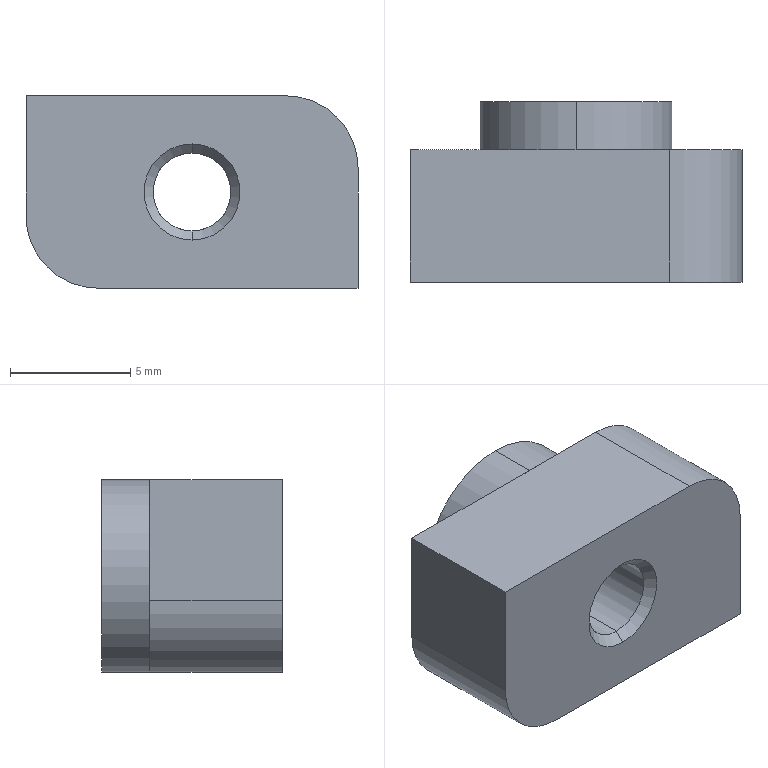Part | SolidWorks | features BaseBody 1 | 1 solid | 18 faces | box 13.8 x 7.5 x 8 mm | volume 622.996 mm3 | plane 8 | cylinder 6 | cone 4 | commonest cylinder face diameters 3.242 x2 6 x2 8 x2
STEP:
#1=CARTESIAN_POINT('',(6.9,0.379,-2.379));
#2=VERTEX_POINT('',#1);
#3=CARTESIAN_POINT('',(6.9,0.379,-5.621));
#4=VERTEX_POINT('',#3);
#5=CARTESIAN_POINT('',(6.9,0.379,-4.));
#6=DIRECTION('',(0.,-1.,0.));
#7=DIRECTION('',(0.,0.,-1.));
#8=AXIS2_PLACEMENT_3D('',#5,#6,#7);
#9=CIRCLE('',#8,1.621);
#10=EDGE_CURVE('',#2,#4,#9,.T.);
#11=ORIENTED_EDGE('',*,*,#10,.F.);
#12=CARTESIAN_POINT('',(6.9,0.,-2.));
#13=VERTEX_POINT('',#12);
#14=CARTESIAN_POINT('',(6.9,0.,-2.));
#15=DIRECTION('',(0.,-0.7071,0.7071));
#16=VECTOR('',#15,1000.);
#17=LINE('',#14,#16);
#18=EDGE_CURVE('',#2,#13,#17,.T.);
#19=ORIENTED_EDGE('',*,*,#18,.T.);
#20=CARTESIAN_POINT('',(6.9,0.,-6.));
#21=VERTEX_POINT('',#20);
#22=CARTESIAN_POINT('',(6.9,0.,-4.));
#23=DIRECTION('',(0.,-1.,0.));
#24=DIRECTION('',(0.,0.,-1.));
#25=AXIS2_PLACEMENT_3D('',#22,#23,#24);
#26=CIRCLE('',#25,2.);
#27=EDGE_CURVE('',#13,#21,#26,.T.);
#28=ORIENTED_EDGE('',*,*,#27,.T.);
#29=CARTESIAN_POINT('',(6.9,0.,-6.));
#30=DIRECTION('',(0.,-0.7071,-0.7071));
#31=VECTOR('',#30,1000.);
#32=LINE('',#29,#31);
#33=EDGE_CURVE('',#4,#21,#32,.T.);
#34=ORIENTED_EDGE('',*,*,#33,.F.);
#35=EDGE_LOOP('',(#11,#19,#28,#34));
#36=FACE_OUTER_BOUND('',#35,.T.);
#37=CARTESIAN_POINT('',(6.9,0.,-4.));
#38=DIRECTION('',(0.,-1.,0.));
#39=DIRECTION('',(0.,0.,-1.));
#40=AXIS2_PLACEMENT_3D('',#37,#38,#39);
#41=CONICAL_SURFACE('',#40,2.,0.7854);
#42=ADVANCED_FACE('',(#36),#41,.F.);
#43=ORIENTED_EDGE('',*,*,#10,.T.);
#44=CARTESIAN_POINT('',(6.9,7.121,-5.621));
#45=VERTEX_POINT('',#44);
#46=CARTESIAN_POINT('',(6.9,0.,-5.621));
#47=DIRECTION('',(0.,1.,0.));
#48=VECTOR('',#47,1000.);
#49=LINE('',#46,#48);
#50=EDGE_CURVE('',#4,#45,#49,.T.);
#51=ORIENTED_EDGE('',*,*,#50,.T.);
#52=CARTESIAN_POINT('',(5.279,7.121,-4.));
#53=VERTEX_POINT('',#52);
#54=CARTESIAN_POINT('',(6.9,7.121,-4.));
#55=DIRECTION('',(0.,-1.,0.));
#56=DIRECTION('',(0.,0.,1.));
#57=AXIS2_PLACEMENT_3D('',#54,#55,#56);
#58=CIRCLE('',#57,1.621);
#59=EDGE_CURVE('',#53,#45,#58,.T.);
#60=ORIENTED_EDGE('',*,*,#59,.F.);
#61=CARTESIAN_POINT('',(6.9,7.121,-2.379));
#62=VERTEX_POINT('',#61);
#63=CARTESIAN_POINT('',(6.9,7.121,-4.));
#64=DIRECTION('',(0.,-1.,0.));
#65=DIRECTION('',(0.,0.,1.));
#66=AXIS2_PLACEMENT_3D('',#63,#64,#65);
#67=CIRCLE('',#66,1.621);
#68=EDGE_CURVE('',#62,#53,#67,.T.);
#69=ORIENTED_EDGE('',*,*,#68,.F.);
#70=CARTESIAN_POINT('',(6.9,0.,-2.379));
#71=DIRECTION('',(0.,1.,0.));
#72=VECTOR('',#71,1000.);
#73=LINE('',#70,#72);
#74=EDGE_CURVE('',#2,#62,#73,.T.);
#75=ORIENTED_EDGE('',*,*,#74,.F.);
#76=EDGE_LOOP('',(#43,#51,#60,#69,#75));
#77=FACE_OUTER_BOUND('',#76,.T.);
#78=CARTESIAN_POINT('',(6.9,0.,-4.));
#79=DIRECTION('',(0.,1.,0.));
#80=DIRECTION('',(0.,0.,1.));
#81=AXIS2_PLACEMENT_3D('',#78,#79,#80);
#82=CYLINDRICAL_SURFACE('',#81,1.621);
#83=ADVANCED_FACE('',(#77),#82,.F.);
#84=ORIENTED_EDGE('',*,*,#59,.T.);
#85=CARTESIAN_POINT('',(8.521,7.121,-4.));
#86=VERTEX_POINT('',#85);
#87=CARTESIAN_POINT('',(6.9,7.121,-4.));
#88=DIRECTION('',(0.,-1.,0.));
#89=DIRECTION('',(0.,0.,1.));
#90=AXIS2_PLACEMENT_3D('',#87,#88,#89);
#91=CIRCLE('',#90,1.621);
#92=EDGE_CURVE('',#45,#86,#91,.T.);
#93=ORIENTED_EDGE('',*,*,#92,.T.);
#94=CARTESIAN_POINT('',(8.9,7.5,-4.));
#95=VERTEX_POINT('',#94);
#96=CARTESIAN_POINT('',(8.9,7.5,-4.));
#97=DIRECTION('',(0.7071,0.7071,0.));
#98=VECTOR('',#97,1000.);
#99=LINE('',#96,#98);
#100=EDGE_CURVE('',#86,#95,#99,.T.);
#101=ORIENTED_EDGE('',*,*,#100,.T.);
#102=CARTESIAN_POINT('',(4.9,7.5,-4.));
#103=VERTEX_POINT('',#102);
#104=CARTESIAN_POINT('',(6.9,7.5,-4.));
#105=DIRECTION('',(0.,-1.,0.));
#106=DIRECTION('',(-1.,0.,0.));
#107=AXIS2_PLACEMENT_3D('',#104,#105,#106);
#108=CIRCLE('',#107,2.);
#109=EDGE_CURVE('',#103,#95,#108,.T.);
#110=ORIENTED_EDGE('',*,*,#109,.F.);
#111=CARTESIAN_POINT('',(4.9,7.5,-4.));
#112=DIRECTION('',(-0.7071,0.7071,0.));
#113=VECTOR('',#112,1000.);
#114=LINE('',#111,#113);
#115=EDGE_CURVE('',#53,#103,#114,.T.);
#116=ORIENTED_EDGE('',*,*,#115,.F.);
#117=EDGE_LOOP('',(#84,#93,#101,#110,#116));
#118=FACE_OUTER_BOUND('',#117,.T.);
#119=CARTESIAN_POINT('',(6.9,7.5,-4.));
#120=DIRECTION('',(0.,1.,0.));
#121=DIRECTION('',(-1.,0.,0.));
#122=AXIS2_PLACEMENT_3D('',#119,#120,#121);
#123=CONICAL_SURFACE('',#122,2.,0.7854);
#124=ADVANCED_FACE('',(#118),#123,.F.);
#125=CARTESIAN_POINT('',(6.9,5.5,-8.));
#126=VERTEX_POINT('',#125);
#127=CARTESIAN_POINT('',(6.9,5.5,0.));
#128=VERTEX_POINT('',#127);
#129=CARTESIAN_POINT('',(6.9,5.5,-4.));
#130=DIRECTION('',(0.,-1.,0.));
#131=DIRECTION('',(0.,0.,1.));
#132=AXIS2_PLACEMENT_3D('',#129,#130,#131);
#133=CIRCLE('',#132,4.);
#134=EDGE_CURVE('',#126,#128,#133,.T.);
#135=ORIENTED_EDGE('',*,*,#134,.F.);
#136=CARTESIAN_POINT('',(6.9,7.5,-8.));
#137=VERTEX_POINT('',#136);
#138=CARTESIAN_POINT('',(6.9,7.5,-8.));
#139=DIRECTION('',(0.,1.,0.));
#140=VECTOR('',#139,1000.);
#141=LINE('',#138,#140);
#142=EDGE_CURVE('',#126,#137,#141,.T.);
#143=ORIENTED_EDGE('',*,*,#142,.T.);
#144=CARTESIAN_POINT('',(6.9,7.5,0.));
#145=VERTEX_POINT('',#144);
#146=CARTESIAN_POINT('',(6.9,7.5,-4.));
#147=DIRECTION('',(0.,-1.,0.));
#148=DIRECTION('',(0.,0.,1.));
#149=AXIS2_PLACEMENT_3D('',#146,#147,#148);
#150=CIRCLE('',#149,4.);
#151=EDGE_CURVE('',#137,#145,#150,.T.);
#152=ORIENTED_EDGE('',*,*,#151,.T.);
#153=CARTESIAN_POINT('',(6.9,7.5,0.));
#154=DIRECTION('',(0.,1.,0.));
#155=VECTOR('',#154,1000.);
#156=LINE('',#153,#155);
#157=EDGE_CURVE('',#128,#145,#156,.T.);
#158=ORIENTED_EDGE('',*,*,#157,.F.);
#159=EDGE_LOOP('',(#135,#143,#152,#158));
#160=FACE_OUTER_BOUND('',#159,.T.);
#161=CARTESIAN_POINT('',(6.9,7.5,-4.));
#162=DIRECTION('',(0.,1.,0.));
#163=DIRECTION('',(0.,0.,1.));
#164=AXIS2_PLACEMENT_3D('',#161,#162,#163);
#165=CYLINDRICAL_SURFACE('',#164,4.);
#166=ADVANCED_FACE('',(#160),#165,.T.);
#167=CARTESIAN_POINT('',(6.9,0.,-4.));
#168=DIRECTION('',(0.,-1.,0.));
#169=DIRECTION('',(0.,0.,-1.));
#170=AXIS2_PLACEMENT_3D('',#167,#168,#169);
#171=CIRCLE('',#170,2.);
#172=EDGE_CURVE('',#21,#13,#171,.T.);
#173=ORIENTED_EDGE('',*,*,#172,.F.);
#174=ORIENTED_EDGE('',*,*,#27,.F.);
#175=EDGE_LOOP('',(#173,#174));
#176=FACE_BOUND('',#175,.T.);
#177=CARTESIAN_POINT('',(0.,0.,0.));
#178=VERTEX_POINT('',#177);
#179=CARTESIAN_POINT('',(10.8,0.,0.));
#180=VERTEX_POINT('',#179);
#181=CARTESIAN_POINT('',(10.8,0.,0.));
#182=DIRECTION('',(1.,0.,0.));
#183=VECTOR('',#182,1000.);
#184=LINE('',#181,#183);
#185=EDGE_CURVE('',#178,#180,#184,.T.);
#186=ORIENTED_EDGE('',*,*,#185,.F.);
#187=CARTESIAN_POINT('',(0.,0.,-5.));
#188=VERTEX_POINT('',#187);
#189=CARTESIAN_POINT('',(0.,0.,-3.));
#190=DIRECTION('',(0.,0.,1.));
#191=VECTOR('',#190,1000.);
#192=LINE('',#189,#191);
#193=EDGE_CURVE('',#188,#178,#192,.T.);
#194=ORIENTED_EDGE('',*,*,#193,.F.);
#195=CARTESIAN_POINT('',(3.,0.,-8.));
#196=VERTEX_POINT('',#195);
#197=CARTESIAN_POINT('',(3.,0.,-5.));
#198=DIRECTION('',(0.,1.,0.));
#199=DIRECTION('',(0.,0.,1.));
#200=AXIS2_PLACEMENT_3D('',#197,#198,#199);
#201=CIRCLE('',#200,3.);
#202=EDGE_CURVE('',#196,#188,#201,.T.);
#203=ORIENTED_EDGE('',*,*,#202,.F.);
#204=CARTESIAN_POINT('',(13.8,0.,-8.));
#205=VERTEX_POINT('',#204);
#206=CARTESIAN_POINT('',(10.8,0.,-8.));
#207=DIRECTION('',(-1.,0.,0.));
#208=VECTOR('',#207,1000.);
#209=LINE('',#206,#208);
#210=EDGE_CURVE('',#205,#196,#209,.T.);
#211=ORIENTED_EDGE('',*,*,#210,.F.);
#212=CARTESIAN_POINT('',(13.8,0.,-3.));
#213=VERTEX_POINT('',#212);
#214=CARTESIAN_POINT('',(13.8,0.,-3.));
#215=DIRECTION('',(0.,0.,-1.));
#216=VECTOR('',#215,1000.);
#217=LINE('',#214,#216);
#218=EDGE_CURVE('',#213,#205,#217,.T.);
#219=ORIENTED_EDGE('',*,*,#218,.F.);
#220=CARTESIAN_POINT('',(10.8,0.,-3.));
#221=DIRECTION('',(0.,1.,0.));
#222=DIRECTION('',(0.,0.,1.));
#223=AXIS2_PLACEMENT_3D('',#220,#221,#222);
#224=CIRCLE('',#223,3.);
#225=EDGE_CURVE('',#180,#213,#224,.T.);
#226=ORIENTED_EDGE('',*,*,#225,.F.);
#227=EDGE_LOOP('',(#186,#194,#203,#211,#219,#226));
#228=FACE_OUTER_BOUND('',#227,.T.);
#229=CARTESIAN_POINT('',(10.8,0.,-3.));
#230=DIRECTION('',(0.,1.,0.));
#231=DIRECTION('',(0.,0.,1.));
#232=AXIS2_PLACEMENT_3D('',#229,#230,#231);
#233=PLANE('',#232);
#234=ADVANCED_FACE('',(#176,#228),#233,.F.);
#235=ORIENTED_EDGE('',*,*,#18,.F.);
#236=CARTESIAN_POINT('',(6.9,0.379,-4.));
#237=DIRECTION('',(0.,-1.,0.));
#238=DIRECTION('',(0.,0.,-1.));
#239=AXIS2_PLACEMENT_3D('',#236,#237,#238);
#240=CIRCLE('',#239,1.621);
#241=EDGE_CURVE('',#4,#2,#240,.T.);
#242=ORIENTED_EDGE('',*,*,#241,.F.);
#243=ORIENTED_EDGE('',*,*,#33,.T.);
#244=ORIENTED_EDGE('',*,*,#172,.T.);
#245=EDGE_LOOP('',(#235,#242,#243,#244));
#246=FACE_OUTER_BOUND('',#245,.T.);
#247=CARTESIAN_POINT('',(6.9,0.,-4.));
#248=DIRECTION('',(0.,-1.,0.));
#249=DIRECTION('',(0.,0.,-1.));
#250=AXIS2_PLACEMENT_3D('',#247,#248,#249);
#251=CONICAL_SURFACE('',#250,2.,0.7854);
#252=ADVANCED_FACE('',(#246),#251,.F.);
#253=CARTESIAN_POINT('',(13.8,5.5,-3.));
#254=VERTEX_POINT('',#253);
#255=CARTESIAN_POINT('',(10.8,5.5,0.));
#256=VERTEX_POINT('',#255);
#257=CARTESIAN_POINT('',(10.8,5.5,-3.));
#258=DIRECTION('',(0.,-1.,0.));
#259=DIRECTION('',(0.,0.,1.));
#260=AXIS2_PLACEMENT_3D('',#257,#258,#259);
#261=CIRCLE('',#260,3.);
#262=EDGE_CURVE('',#254,#256,#261,.T.);
#263=ORIENTED_EDGE('',*,*,#262,.T.);
#264=CARTESIAN_POINT('',(10.8,5.5,0.));
#265=DIRECTION('',(0.,-1.,0.));
#266=VECTOR('',#265,1000.);
#267=LINE('',#264,#266);
#268=EDGE_CURVE('',#256,#180,#267,.T.);
#269=ORIENTED_EDGE('',*,*,#268,.T.);
#270=ORIENTED_EDGE('',*,*,#225,.T.);
#271=CARTESIAN_POINT('',(13.8,5.5,-3.));
#272=DIRECTION('',(0.,1.,0.));
#273=VECTOR('',#272,1000.);
#274=LINE('',#271,#273);
#275=EDGE_CURVE('',#213,#254,#274,.T.);
#276=ORIENTED_EDGE('',*,*,#275,.T.);
#277=EDGE_LOOP('',(#263,#269,#270,#276));
#278=FACE_OUTER_BOUND('',#277,.T.);
#279=CARTESIAN_POINT('',(10.8,5.5,-3.));
#280=DIRECTION('',(0.,1.,0.));
#281=DIRECTION('',(0.,0.,1.));
#282=AXIS2_PLACEMENT_3D('',#279,#280,#281);
#283=CYLINDRICAL_SURFACE('',#282,3.);
#284=ADVANCED_FACE('',(#278),#283,.T.);
#285=ORIENTED_EDGE('',*,*,#268,.F.);
#286=CARTESIAN_POINT('',(0.,5.5,0.));
#287=DIRECTION('',(1.,0.,0.));
#288=VECTOR('',#287,1000.);
#289=LINE('',#286,#288);
#290=EDGE_CURVE('',#128,#256,#289,.T.);
#291=ORIENTED_EDGE('',*,*,#290,.F.);
#292=CARTESIAN_POINT('',(0.,5.5,0.));
#293=VERTEX_POINT('',#292);
#294=CARTESIAN_POINT('',(0.,5.5,0.));
#295=DIRECTION('',(1.,0.,0.));
#296=VECTOR('',#295,1000.);
#297=LINE('',#294,#296);
#298=EDGE_CURVE('',#293,#128,#297,.T.);
#299=ORIENTED_EDGE('',*,*,#298,.F.);
#300=CARTESIAN_POINT('',(0.,5.5,0.));
#301=DIRECTION('',(0.,1.,0.));
#302=VECTOR('',#301,1000.);
#303=LINE('',#300,#302);
#304=EDGE_CURVE('',#178,#293,#303,.T.);
#305=ORIENTED_EDGE('',*,*,#304,.F.);
#306=ORIENTED_EDGE('',*,*,#185,.T.);
#307=EDGE_LOOP('',(#285,#291,#299,#305,#306));
#308=FACE_OUTER_BOUND('',#307,.T.);
#309=CARTESIAN_POINT('',(0.,5.5,0.));
#310=DIRECTION('',(0.,0.,-1.));
#311=DIRECTION('',(-1.,0.,0.));
#312=AXIS2_PLACEMENT_3D('',#309,#310,#311);
#313=PLANE('',#312);
#314=ADVANCED_FACE('',(#308),#313,.F.);
#315=ORIENTED_EDGE('',*,*,#304,.T.);
#316=CARTESIAN_POINT('',(0.,5.5,-5.));
#317=VERTEX_POINT('',#316);
#318=CARTESIAN_POINT('',(0.,5.5,-5.));
#319=DIRECTION('',(0.,0.,1.));
#320=VECTOR('',#319,1000.);
#321=LINE('',#318,#320);
#322=EDGE_CURVE('',#317,#293,#321,.T.);
#323=ORIENTED_EDGE('',*,*,#322,.F.);
#324=CARTESIAN_POINT('',(0.,5.5,-5.));
#325=DIRECTION('',(0.,1.,0.));
#326=VECTOR('',#325,1000.);
#327=LINE('',#324,#326);
#328=EDGE_CURVE('',#188,#317,#327,.T.);
#329=ORIENTED_EDGE('',*,*,#328,.F.);
#330=ORIENTED_EDGE('',*,*,#193,.T.);
#331=EDGE_LOOP('',(#315,#323,#329,#330));
#332=FACE_OUTER_BOUND('',#331,.T.);
#333=CARTESIAN_POINT('',(0.,5.5,-5.));
#334=DIRECTION('',(1.,0.,0.));
#335=DIRECTION('',(0.,0.,-1.));
#336=AXIS2_PLACEMENT_3D('',#333,#334,#335);
#337=PLANE('',#336);
#338=ADVANCED_FACE('',(#332),#337,.F.);
#339=CARTESIAN_POINT('',(3.,5.5,-8.));
#340=VERTEX_POINT('',#339);
#341=CARTESIAN_POINT('',(3.,5.5,-5.));
#342=DIRECTION('',(0.,-1.,0.));
#343=DIRECTION('',(0.,0.,1.));
#344=AXIS2_PLACEMENT_3D('',#341,#342,#343);
#345=CIRCLE('',#344,3.);
#346=EDGE_CURVE('',#317,#340,#345,.T.);
#347=ORIENTED_EDGE('',*,*,#346,.T.);
#348=CARTESIAN_POINT('',(3.,5.5,-8.));
#349=DIRECTION('',(0.,-1.,0.));
#350=VECTOR('',#349,1000.);
#351=LINE('',#348,#350);
#352=EDGE_CURVE('',#340,#196,#351,.T.);
#353=ORIENTED_EDGE('',*,*,#352,.T.);
#354=ORIENTED_EDGE('',*,*,#202,.T.);
#355=ORIENTED_EDGE('',*,*,#328,.T.);
#356=EDGE_LOOP('',(#347,#353,#354,#355));
#357=FACE_OUTER_BOUND('',#356,.T.);
#358=CARTESIAN_POINT('',(3.,5.5,-5.));
#359=DIRECTION('',(0.,1.,0.));
#360=DIRECTION('',(0.,0.,1.));
#361=AXIS2_PLACEMENT_3D('',#358,#359,#360);
#362=CYLINDRICAL_SURFACE('',#361,3.);
#363=ADVANCED_FACE('',(#357),#362,.T.);
#364=ORIENTED_EDGE('',*,*,#352,.F.);
#365=CARTESIAN_POINT('',(13.8,5.5,-8.));
#366=DIRECTION('',(-1.,0.,0.));
#367=VECTOR('',#366,1000.);
#368=LINE('',#365,#367);
#369=EDGE_CURVE('',#126,#340,#368,.T.);
#370=ORIENTED_EDGE('',*,*,#369,.F.);
#371=CARTESIAN_POINT('',(13.8,5.5,-8.));
#372=VERTEX_POINT('',#371);
#373=CARTESIAN_POINT('',(13.8,5.5,-8.));
#374=DIRECTION('',(-1.,0.,0.));
#375=VECTOR('',#374,1000.);
#376=LINE('',#373,#375);
#377=EDGE_CURVE('',#372,#126,#376,.T.);
#378=ORIENTED_EDGE('',*,*,#377,.F.);
#379=CARTESIAN_POINT('',(13.8,5.5,-8.));
#380=DIRECTION('',(0.,1.,0.));
#381=VECTOR('',#380,1000.);
#382=LINE('',#379,#381);
#383=EDGE_CURVE('',#205,#372,#382,.T.);
#384=ORIENTED_EDGE('',*,*,#383,.F.);
#385=ORIENTED_EDGE('',*,*,#210,.T.);
#386=EDGE_LOOP('',(#364,#370,#378,#384,#385));
#387=FACE_OUTER_BOUND('',#386,.T.);
#388=CARTESIAN_POINT('',(13.8,5.5,-8.));
#389=DIRECTION('',(0.,0.,1.));
#390=DIRECTION('',(1.,0.,0.));
#391=AXIS2_PLACEMENT_3D('',#388,#389,#390);
#392=PLANE('',#391);
#393=ADVANCED_FACE('',(#387),#392,.F.);
#394=ORIENTED_EDGE('',*,*,#383,.T.);
#395=CARTESIAN_POINT('',(13.8,5.5,-3.));
#396=DIRECTION('',(0.,0.,-1.));
#397=VECTOR('',#396,1000.);
#398=LINE('',#395,#397);
#399=EDGE_CURVE('',#254,#372,#398,.T.);
#400=ORIENTED_EDGE('',*,*,#399,.F.);
#401=ORIENTED_EDGE('',*,*,#275,.F.);
#402=ORIENTED_EDGE('',*,*,#218,.T.);
#403=EDGE_LOOP('',(#394,#400,#401,#402));
#404=FACE_OUTER_BOUND('',#403,.T.);
#405=CARTESIAN_POINT('',(13.8,5.5,-3.));
#406=DIRECTION('',(-1.,0.,0.));
#407=DIRECTION('',(0.,0.,1.));
#408=AXIS2_PLACEMENT_3D('',#405,#406,#407);
#409=PLANE('',#408);
#410=ADVANCED_FACE('',(#404),#409,.F.);
#411=ORIENTED_EDGE('',*,*,#50,.F.);
#412=ORIENTED_EDGE('',*,*,#241,.T.);
#413=ORIENTED_EDGE('',*,*,#74,.T.);
#414=CARTESIAN_POINT('',(6.9,7.121,-4.));
#415=DIRECTION('',(0.,-1.,0.));
#416=DIRECTION('',(0.,0.,1.));
#417=AXIS2_PLACEMENT_3D('',#414,#415,#416);
#418=CIRCLE('',#417,1.621);
#419=EDGE_CURVE('',#86,#62,#418,.T.);
#420=ORIENTED_EDGE('',*,*,#419,.F.);
#421=ORIENTED_EDGE('',*,*,#92,.F.);
#422=EDGE_LOOP('',(#411,#412,#413,#420,#421));
#423=FACE_OUTER_BOUND('',#422,.T.);
#424=CARTESIAN_POINT('',(6.9,0.,-4.));
#425=DIRECTION('',(0.,1.,0.));
#426=DIRECTION('',(0.,0.,1.));
#427=AXIS2_PLACEMENT_3D('',#424,#425,#426);
#428=CYLINDRICAL_SURFACE('',#427,1.621);
#429=ADVANCED_FACE('',(#423),#428,.F.);
#430=ORIENTED_EDGE('',*,*,#262,.F.);
#431=ORIENTED_EDGE('',*,*,#399,.T.);
#432=ORIENTED_EDGE('',*,*,#377,.T.);
#433=ORIENTED_EDGE('',*,*,#134,.T.);
#434=ORIENTED_EDGE('',*,*,#290,.T.);
#435=EDGE_LOOP('',(#430,#431,#432,#433,#434));
#436=FACE_OUTER_BOUND('',#435,.T.);
#437=CARTESIAN_POINT('',(10.8,5.5,-3.));
#438=DIRECTION('',(0.,1.,0.));
#439=DIRECTION('',(0.,0.,1.));
#440=AXIS2_PLACEMENT_3D('',#437,#438,#439);
#441=PLANE('',#440);
#442=ADVANCED_FACE('',(#436),#441,.T.);
#443=ORIENTED_EDGE('',*,*,#346,.F.);
#444=ORIENTED_EDGE('',*,*,#322,.T.);
#445=ORIENTED_EDGE('',*,*,#298,.T.);
#446=CARTESIAN_POINT('',(6.9,5.5,-4.));
#447=DIRECTION('',(0.,-1.,0.));
#448=DIRECTION('',(0.,0.,1.));
#449=AXIS2_PLACEMENT_3D('',#446,#447,#448);
#450=CIRCLE('',#449,4.);
#451=EDGE_CURVE('',#128,#126,#450,.T.);
#452=ORIENTED_EDGE('',*,*,#451,.T.);
#453=ORIENTED_EDGE('',*,*,#369,.T.);
#454=EDGE_LOOP('',(#443,#444,#445,#452,#453));
#455=FACE_OUTER_BOUND('',#454,.T.);
#456=CARTESIAN_POINT('',(10.8,5.5,-3.));
#457=DIRECTION('',(0.,1.,0.));
#458=DIRECTION('',(0.,0.,1.));
#459=AXIS2_PLACEMENT_3D('',#456,#457,#458);
#460=PLANE('',#459);
#461=ADVANCED_FACE('',(#455),#460,.T.);
#462=ORIENTED_EDGE('',*,*,#100,.F.);
#463=ORIENTED_EDGE('',*,*,#419,.T.);
#464=ORIENTED_EDGE('',*,*,#68,.T.);
#465=ORIENTED_EDGE('',*,*,#115,.T.);
#466=CARTESIAN_POINT('',(6.9,7.5,-4.));
#467=DIRECTION('',(0.,-1.,0.));
#468=DIRECTION('',(-1.,0.,0.));
#469=AXIS2_PLACEMENT_3D('',#466,#467,#468);
#470=CIRCLE('',#469,2.);
#471=EDGE_CURVE('',#95,#103,#470,.T.);
#472=ORIENTED_EDGE('',*,*,#471,.F.);
#473=EDGE_LOOP('',(#462,#463,#464,#465,#472));
#474=FACE_OUTER_BOUND('',#473,.T.);
#475=CARTESIAN_POINT('',(6.9,7.5,-4.));
#476=DIRECTION('',(0.,1.,0.));
#477=DIRECTION('',(-1.,0.,0.));
#478=AXIS2_PLACEMENT_3D('',#475,#476,#477);
#479=CONICAL_SURFACE('',#478,2.,0.7854);
#480=ADVANCED_FACE('',(#474),#479,.F.);
#481=ORIENTED_EDGE('',*,*,#142,.F.);
#482=ORIENTED_EDGE('',*,*,#451,.F.);
#483=ORIENTED_EDGE('',*,*,#157,.T.);
#484=CARTESIAN_POINT('',(6.9,7.5,-4.));
#485=DIRECTION('',(0.,-1.,0.));
#486=DIRECTION('',(0.,0.,1.));
#487=AXIS2_PLACEMENT_3D('',#484,#485,#486);
#488=CIRCLE('',#487,4.);
#489=EDGE_CURVE('',#145,#137,#488,.T.);
#490=ORIENTED_EDGE('',*,*,#489,.T.);
#491=EDGE_LOOP('',(#481,#482,#483,#490));
#492=FACE_OUTER_BOUND('',#491,.T.);
#493=CARTESIAN_POINT('',(6.9,7.5,-4.));
#494=DIRECTION('',(0.,1.,0.));
#495=DIRECTION('',(0.,0.,1.));
#496=AXIS2_PLACEMENT_3D('',#493,#494,#495);
#497=CYLINDRICAL_SURFACE('',#496,4.);
#498=ADVANCED_FACE('',(#492),#497,.T.);
#499=ORIENTED_EDGE('',*,*,#109,.T.);
#500=ORIENTED_EDGE('',*,*,#471,.T.);
#501=EDGE_LOOP('',(#499,#500));
#502=FACE_BOUND('',#501,.T.);
#503=ORIENTED_EDGE('',*,*,#489,.F.);
#504=ORIENTED_EDGE('',*,*,#151,.F.);
#505=EDGE_LOOP('',(#503,#504));
#506=FACE_OUTER_BOUND('',#505,.T.);
#507=CARTESIAN_POINT('',(6.9,7.5,-4.));
#508=DIRECTION('',(0.,1.,0.));
#509=DIRECTION('',(0.,0.,1.));
#510=AXIS2_PLACEMENT_3D('',#507,#508,#509);
#511=PLANE('',#510);
#512=ADVANCED_FACE('',(#502,#506),#511,.T.);
#513=CLOSED_SHELL('',(#42,#83,#124,#166,#234,#252,#284,#314,#338,#363,#393,#410,#429,#442,#461,#480,#498,#512));
#514=MANIFOLD_SOLID_BREP('',#513);
#515=CARTESIAN_POINT('',(0.,0.,0.));
#516=DIRECTION('',(0.,0.,1.));
#517=DIRECTION('',(1.,0.,0.));
#518=AXIS2_PLACEMENT_3D('',#515,#516,#517);
#519=(LENGTH_UNIT()NAMED_UNIT(*)SI_UNIT(.MILLI.,.METRE.));
#520=UNCERTAINTY_MEASURE_WITH_UNIT(LENGTH_MEASURE(0.00001),#519,'','');
#521=(NAMED_UNIT(*)PLANE_ANGLE_UNIT()SI_UNIT($,.RADIAN.));
#522=(NAMED_UNIT(*)SI_UNIT($,.STERADIAN.)SOLID_ANGLE_UNIT());
#523=(GEOMETRIC_REPRESENTATION_CONTEXT(3)GLOBAL_UNCERTAINTY_ASSIGNED_CONTEXT((#520))GLOBAL_UNIT_ASSIGNED_CONTEXT((#519,#521,#522))REPRESENTATION_CONTEXT('',''));
#524=ADVANCED_BREP_SHAPE_REPRESENTATION('',(#514,#518),#523);